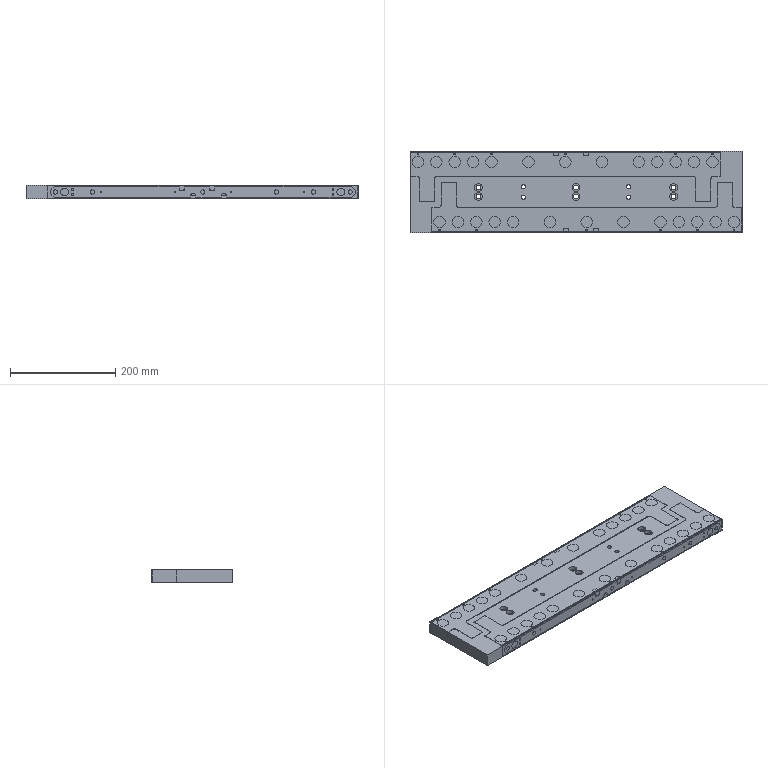NC program | NX | posted with a generic post | part box 631 x 154 x 25 mm
Lines 131 to 967 of 18383:
(HOLE_MILLING_COPY , TOOL : D10JING)
N242 T11 M6
N244 G54
N246 G17 G0 G90 X-200.5 Y47. B0. C0. S7000 M3
N248 G43 Z30. H11
N250 Z1.
N252 G94 G3 X-197.575 Y44.075 R2.925 F2000.
N254 X-194.65 Y47. R2.925
N256 X-194.65 Y47. Z0. I-5.85 J0.
N258 X-194.65 Y47. Z-1. I-5.85 J0.
N260 X-194.65 Y47. Z-2. I-5.85 J0.
N262 X-194.65 Y47. Z-3. I-5.85 J0.
N264 X-194.65 Y47. Z-4. I-5.85 J0.
N266 X-194.65 Y47. Z-5. I-5.85 J0.
N268 X-194.65 Y47. Z-6. I-5.85 J0.
N270 X-200.5 Y52.85 R5.85
N272 X-194.65 Y47. R-5.85
N274 X-197.575 Y49.925 R2.925
N276 X-200.5 Y47. R2.925
N278 G0 Z30.
N280 X-165.5
N282 Z1.
N284 G3 X-162.575 Y44.075 R2.925
N286 X-159.65 Y47. R2.925
N288 X-159.65 Y47. Z0. I-5.85 J0.
N290 X-159.65 Y47. Z-1. I-5.85 J0.
N292 X-159.65 Y47. Z-2. I-5.85 J0.
N294 X-159.65 Y47. Z-3. I-5.85 J0.
N296 X-159.65 Y47. Z-4. I-5.85 J0.
N298 X-159.65 Y47. Z-5. I-5.85 J0.
N300 X-159.65 Y47. Z-6. I-5.85 J0.
N302 X-165.5 Y52.85 R5.85
N304 X-159.65 Y47. R-5.85
N306 X-162.575 Y49.925 R2.925
N308 X-165.5 Y47. R2.925
N310 G0 Z30.
N312 X-130.5
N314 Z1.
N316 G3 X-127.575 Y44.075 R2.925
N318 X-124.65 Y47. R2.925
N320 X-124.65 Y47. Z0. I-5.85 J0.
N322 X-124.65 Y47. Z-1. I-5.85 J0.
N324 X-124.65 Y47. Z-2. I-5.85 J0.
N326 X-124.65 Y47. Z-3. I-5.85 J0.
N328 X-124.65 Y47. Z-4. I-5.85 J0.
N330 X-124.65 Y47. Z-5. I-5.85 J0.
N332 X-124.65 Y47. Z-6. I-5.85 J0.
N334 X-130.5 Y52.85 R5.85
N336 X-124.65 Y47. R-5.85
N338 X-127.575 Y49.925 R2.925
N340 X-130.5 Y47. R2.925
N342 G0 Z30.
N344 X-95.5
N346 Z1.
N348 G3 X-92.575 Y44.075 R2.925
N350 X-89.65 Y47. R2.925
N352 X-89.65 Y47. Z0. I-5.85 J0.
N354 X-89.65 Y47. Z-1. I-5.85 J0.
N356 X-89.65 Y47. Z-2. I-5.85 J0.
N358 X-89.65 Y47. Z-3. I-5.85 J0.
N360 X-89.65 Y47. Z-4. I-5.85 J0.
N362 X-89.65 Y47. Z-5. I-5.85 J0.
N364 X-89.65 Y47. Z-6. I-5.85 J0.
N366 X-95.5 Y52.85 R5.85
N368 X-89.65 Y47. R-5.85
N370 X-92.575 Y49.925 R2.925
N372 X-95.5 Y47. R2.925
N374 G0 Z30.
N376 X-60.5
N378 Z1.
N380 G3 X-57.575 Y44.075 R2.925
N382 X-54.65 Y47. R2.925
N384 X-54.65 Y47. Z0. I-5.85 J0.
N386 X-54.65 Y47. Z-1. I-5.85 J0.
N388 X-54.65 Y47. Z-2. I-5.85 J0.
N390 X-54.65 Y47. Z-3. I-5.85 J0.
N392 X-54.65 Y47. Z-4. I-5.85 J0.
N394 X-54.65 Y47. Z-5. I-5.85 J0.
N396 X-54.65 Y47. Z-6. I-5.85 J0.
N398 X-60.5 Y52.85 R5.85
N400 X-54.65 Y47. R-5.85
N402 X-57.575 Y49.925 R2.925
N404 X-60.5 Y47. R2.925
N406 G0 Z30.
N408 X9.5
N410 Z1.
N412 G3 X12.425 Y44.075 R2.925
N414 X15.35 Y47. R2.925
N416 X15.35 Y47. Z0. I-5.85 J0.
N418 X15.35 Y47. Z-1. I-5.85 J0.
N420 X15.35 Y47. Z-2. I-5.85 J0.
N422 X15.35 Y47. Z-3. I-5.85 J0.
N424 X15.35 Y47. Z-4. I-5.85 J0.
N426 X15.35 Y47. Z-5. I-5.85 J0.
N428 X15.35 Y47. Z-6. I-5.85 J0.
N430 X9.5 Y52.85 R5.85
N432 X15.35 Y47. R-5.85
N434 X12.425 Y49.925 R2.925
N436 X9.5 Y47. R2.925
N438 G0 Z30.
N440 X79.5
N442 Z1.
N444 G3 X82.425 Y44.075 R2.925
N446 X85.35 Y47. R2.925
N448 X85.35 Y47. Z0. I-5.85 J0.
N450 X85.35 Y47. Z-1. I-5.85 J0.
N452 X85.35 Y47. Z-2. I-5.85 J0.
N454 X85.35 Y47. Z-3. I-5.85 J0.
N456 X85.35 Y47. Z-4. I-5.85 J0.
N458 X85.35 Y47. Z-5. I-5.85 J0.
N460 X85.35 Y47. Z-6. I-5.85 J0.
N462 X79.5 Y52.85 R5.85
N464 X85.35 Y47. R-5.85
N466 X82.425 Y49.925 R2.925
N468 X79.5 Y47. R2.925
N470 G0 Z30.
N472 X149.5
N474 Z1.
N476 G3 X152.425 Y44.075 R2.925
N478 X155.35 Y47. R2.925
N480 X155.35 Y47. Z0. I-5.85 J0.
N482 X155.35 Y47. Z-1. I-5.85 J0.
N484 X155.35 Y47. Z-2. I-5.85 J0.
N486 X155.35 Y47. Z-3. I-5.85 J0.
N488 X155.35 Y47. Z-4. I-5.85 J0.
N490 X155.35 Y47. Z-5. I-5.85 J0.
N492 X155.35 Y47. Z-6. I-5.85 J0.
N494 X149.5 Y52.85 R5.85
N496 X155.35 Y47. R-5.85
N498 X152.425 Y49.925 R2.925
N500 X149.5 Y47. R2.925
N502 G0 Z30.
N504 X219.5
N506 Z1.
N508 G3 X222.425 Y44.075 R2.925
N510 X225.35 Y47. R2.925
N512 X225.35 Y47. Z0. I-5.85 J0.
N514 X225.35 Y47. Z-1. I-5.85 J0.
N516 X225.35 Y47. Z-2. I-5.85 J0.
N518 X225.35 Y47. Z-3. I-5.85 J0.
N520 X225.35 Y47. Z-4. I-5.85 J0.
N522 X225.35 Y47. Z-5. I-5.85 J0.
N524 X225.35 Y47. Z-6. I-5.85 J0.
N526 X219.5 Y52.85 R5.85
N528 X225.35 Y47. R-5.85
N530 X222.425 Y49.925 R2.925
N532 X219.5 Y47. R2.925
N534 G0 Z30.
N536 X254.5
N538 Z1.
N540 G3 X257.425 Y44.075 R2.925
N542 X260.35 Y47. R2.925
N544 X260.35 Y47. Z0. I-5.85 J0.
N546 X260.35 Y47. Z-1. I-5.85 J0.
N548 X260.35 Y47. Z-2. I-5.85 J0.
N550 X260.35 Y47. Z-3. I-5.85 J0.
N552 X260.35 Y47. Z-4. I-5.85 J0.
N554 X260.35 Y47. Z-5. I-5.85 J0.
N556 X260.35 Y47. Z-6. I-5.85 J0.
N558 X254.5 Y52.85 R5.85
N560 X260.35 Y47. R-5.85
N562 X257.425 Y49.925 R2.925
N564 X254.5 Y47. R2.925
N566 G0 Z30.
N568 X289.5
N570 Z1.
N572 G3 X292.425 Y44.075 R2.925
N574 X295.35 Y47. R2.925
N576 X295.35 Y47. Z0. I-5.85 J0.
N578 X295.35 Y47. Z-1. I-5.85 J0.
N580 X295.35 Y47. Z-2. I-5.85 J0.
N582 X295.35 Y47. Z-3. I-5.85 J0.
N584 X295.35 Y47. Z-4. I-5.85 J0.
N586 X295.35 Y47. Z-5. I-5.85 J0.
N588 X295.35 Y47. Z-6. I-5.85 J0.
N590 X289.5 Y52.85 R5.85
N592 X295.35 Y47. R-5.85
N594 X292.425 Y49.925 R2.925
N596 X289.5 Y47. R2.925
N598 G0 Z30.
N600 X324.5
N602 Z1.
N604 G3 X327.425 Y44.075 R2.925
N606 X330.35 Y47. R2.925
N608 X330.35 Y47. Z0. I-5.85 J0.
N610 X330.35 Y47. Z-1. I-5.85 J0.
N612 X330.35 Y47. Z-2. I-5.85 J0.
N614 X330.35 Y47. Z-3. I-5.85 J0.
N616 X330.35 Y47. Z-4. I-5.85 J0.
N618 X330.35 Y47. Z-5. I-5.85 J0.
N620 X330.35 Y47. Z-6. I-5.85 J0.
N622 X324.5 Y52.85 R5.85
N624 X330.35 Y47. R-5.85
N626 X327.425 Y49.925 R2.925
N628 X324.5 Y47. R2.925
N630 G0 Z30.
N632 X359.5
N634 Z1.
N636 G3 X362.425 Y44.075 R2.925
N638 X365.35 Y47. R2.925
N640 X365.35 Y47. Z0. I-5.85 J0.
N642 X365.35 Y47. Z-1. I-5.85 J0.
N644 X365.35 Y47. Z-2. I-5.85 J0.
N646 X365.35 Y47. Z-3. I-5.85 J0.
N648 X365.35 Y47. Z-4. I-5.85 J0.
N650 X365.35 Y47. Z-5. I-5.85 J0.
N652 X365.35 Y47. Z-6. I-5.85 J0.
N654 X359.5 Y52.85 R5.85
N656 X365.35 Y47. R-5.85
N658 X362.425 Y49.925 R2.925
N660 X359.5 Y47. R2.925
N662 G0 Z30.
N664 X400.5 Y-67.
N666 Z1.
N668 G3 X403.425 Y-69.925 R2.925
N670 X406.35 Y-67. R2.925
N672 X406.35 Y-67. Z0. I-5.85 J0.
N674 X406.35 Y-67. Z-1. I-5.85 J0.
N676 X406.35 Y-67. Z-2. I-5.85 J0.
N678 X406.35 Y-67. Z-3. I-5.85 J0.
N680 X406.35 Y-67. Z-4. I-5.85 J0.
N682 X406.35 Y-67. Z-5. I-5.85 J0.
N684 X406.35 Y-67. Z-6. I-5.85 J0.
N686 X400.5 Y-61.15 R5.85
N688 X406.35 Y-67. R-5.85
N690 X403.425 Y-64.075 R2.925
N692 X400.5 Y-67. R2.925
N694 G0 Z30.
N696 X365.5
N698 Z1.
N700 G3 X368.425 Y-69.925 R2.925
N702 X371.35 Y-67. R2.925
N704 X371.35 Y-67. Z0. I-5.85 J0.
N706 X371.35 Y-67. Z-1. I-5.85 J0.
N708 X371.35 Y-67. Z-2. I-5.85 J0.
N710 X371.35 Y-67. Z-3. I-5.85 J0.
N712 X371.35 Y-67. Z-4. I-5.85 J0.
N714 X371.35 Y-67. Z-5. I-5.85 J0.
N716 X371.35 Y-67. Z-6. I-5.85 J0.
N718 X365.5 Y-61.15 R5.85
N720 X371.35 Y-67. R-5.85
N722 X368.425 Y-64.075 R2.925
N724 X365.5 Y-67. R2.925
N726 G0 Z30.
N728 X330.5
N730 Z1.
N732 G3 X333.425 Y-69.925 R2.925
N734 X336.35 Y-67. R2.925
N736 X336.35 Y-67. Z0. I-5.85 J0.
N738 X336.35 Y-67. Z-1. I-5.85 J0.
N740 X336.35 Y-67. Z-2. I-5.85 J0.
N742 X336.35 Y-67. Z-3. I-5.85 J0.
N744 X336.35 Y-67. Z-4. I-5.85 J0.
N746 X336.35 Y-67. Z-5. I-5.85 J0.
N748 X336.35 Y-67. Z-6. I-5.85 J0.
N750 X330.5 Y-61.15 R5.85
N752 X336.35 Y-67. R-5.85
N754 X333.425 Y-64.075 R2.925
N756 X330.5 Y-67. R2.925
N758 G0 Z30.
N760 X295.5
N762 Z1.
N764 G3 X298.425 Y-69.925 R2.925
N766 X301.35 Y-67. R2.925
N768 X301.35 Y-67. Z0. I-5.85 J0.
N770 X301.35 Y-67. Z-1. I-5.85 J0.
N772 X301.35 Y-67. Z-2. I-5.85 J0.
N774 X301.35 Y-67. Z-3. I-5.85 J0.
N776 X301.35 Y-67. Z-4. I-5.85 J0.
N778 X301.35 Y-67. Z-5. I-5.85 J0.
N780 X301.35 Y-67. Z-6. I-5.85 J0.
N782 X295.5 Y-61.15 R5.85
N784 X301.35 Y-67. R-5.85
N786 X298.425 Y-64.075 R2.925
N788 X295.5 Y-67. R2.925
N790 G0 Z30.
N792 X260.5
N794 Z1.
N796 G3 X263.425 Y-69.925 R2.925
N798 X266.35 Y-67. R2.925
N800 X266.35 Y-67. Z0. I-5.85 J0.
N802 X266.35 Y-67. Z-1. I-5.85 J0.
N804 X266.35 Y-67. Z-2. I-5.85 J0.
N806 X266.35 Y-67. Z-3. I-5.85 J0.
N808 X266.35 Y-67. Z-4. I-5.85 J0.
N810 X266.35 Y-67. Z-5. I-5.85 J0.
N812 X266.35 Y-67. Z-6. I-5.85 J0.
N814 X260.5 Y-61.15 R5.85
N816 X266.35 Y-67. R-5.85
N818 X263.425 Y-64.075 R2.925
N820 X260.5 Y-67. R2.925
N822 G0 Z30.
N824 X190.5
N826 Z1.
N828 G3 X193.425 Y-69.925 R2.925
N830 X196.35 Y-67. R2.925
N832 X196.35 Y-67. Z0. I-5.85 J0.
N834 X196.35 Y-67. Z-1. I-5.85 J0.
N836 X196.35 Y-67. Z-2. I-5.85 J0.
N838 X196.35 Y-67. Z-3. I-5.85 J0.
N840 X196.35 Y-67. Z-4. I-5.85 J0.
N842 X196.35 Y-67. Z-5. I-5.85 J0.
N844 X196.35 Y-67. Z-6. I-5.85 J0.
N846 X190.5 Y-61.15 R5.85
N848 X196.35 Y-67. R-5.85
N850 X193.425 Y-64.075 R2.925
N852 X190.5 Y-67. R2.925
N854 G0 Z30.
N856 X120.5
N858 Z1.
N860 G3 X123.425 Y-69.925 R2.925
N862 X126.35 Y-67. R2.925
N864 X126.35 Y-67. Z0. I-5.85 J0.
N866 X126.35 Y-67. Z-1. I-5.85 J0.
N868 X126.35 Y-67. Z-2. I-5.85 J0.
N870 X126.35 Y-67. Z-3. I-5.85 J0.
N872 X126.35 Y-67. Z-4. I-5.85 J0.
N874 X126.35 Y-67. Z-5. I-5.85 J0.
N876 X126.35 Y-67. Z-6. I-5.85 J0.
N878 X120.5 Y-61.15 R5.85
N880 X126.35 Y-67. R-5.85
N882 X123.425 Y-64.075 R2.925
N884 X120.5 Y-67. R2.925
N886 G0 Z30.
N888 X50.5
N890 Z1.
N892 G3 X53.425 Y-69.925 R2.925
N894 X56.35 Y-67. R2.925
N896 X56.35 Y-67. Z0. I-5.85 J0.
N898 X56.35 Y-67. Z-1. I-5.85 J0.
N900 X56.35 Y-67. Z-2. I-5.85 J0.
N902 X56.35 Y-67. Z-3. I-5.85 J0.
N904 X56.35 Y-67. Z-4. I-5.85 J0.
N906 X56.35 Y-67. Z-5. I-5.85 J0.
N908 X56.35 Y-67. Z-6. I-5.85 J0.
N910 X50.5 Y-61.15 R5.85
N912 X56.35 Y-67. R-5.85
N914 X53.425 Y-64.075 R2.925
N916 X50.5 Y-67. R2.925
N918 G0 Z30.
N920 X-19.5
N922 Z1.
N924 G3 X-16.575 Y-69.925 R2.925
N926 X-13.65 Y-67. R2.925
N928 X-13.65 Y-67. Z0. I-5.85 J0.
N930 X-13.65 Y-67. Z-1. I-5.85 J0.
N932 X-13.65 Y-67. Z-2. I-5.85 J0.
N934 X-13.65 Y-67. Z-3. I-5.85 J0.
N936 X-13.65 Y-67. Z-4. I-5.85 J0.
N938 X-13.65 Y-67. Z-5. I-5.85 J0.
N940 X-13.65 Y-67. Z-6. I-5.85 J0.
N942 X-19.5 Y-61.15 R5.85
N944 X-13.65 Y-67. R-5.85
N946 X-16.575 Y-64.075 R2.925
N948 X-19.5 Y-67. R2.925
N950 G0 Z30.
N952 X-54.5
N954 Z1.
N956 G3 X-51.575 Y-69.925 R2.925
N958 X-48.65 Y-67. R2.925
N960 X-48.65 Y-67. Z0. I-5.85 J0.
N962 X-48.65 Y-67. Z-1. I-5.85 J0.
N964 X-48.65 Y-67. Z-2. I-5.85 J0.
N966 X-48.65 Y-67. Z-3. I-5.85 J0.
N968 X-48.65 Y-67. Z-4. I-5.85 J0.
N970 X-48.65 Y-67. Z-5. I-5.85 J0.
N972 X-48.65 Y-67. Z-6. I-5.85 J0.
N974 X-54.5 Y-61.15 R5.85
N976 X-48.65 Y-67. R-5.85
N978 X-51.575 Y-64.075 R2.925
N980 X-54.5 Y-67. R2.925
N982 G0 Z30.
N984 X-89.5
N986 Z1.
N988 G3 X-86.575 Y-69.925 R2.925
N990 X-83.65 Y-67. R2.925
N992 X-83.65 Y-67. Z0. I-5.85 J0.
N994 X-83.65 Y-67. Z-1. I-5.85 J0.
N996 X-83.65 Y-67. Z-2. I-5.85 J0.
N998 X-83.65 Y-67. Z-3. I-5.85 J0.
N1000 X-83.65 Y-67. Z-4. I-5.85 J0.
N1002 X-83.65 Y-67. Z-5. I-5.85 J0.
N1004 X-83.65 Y-67. Z-6. I-5.85 J0.
N1006 X-89.5 Y-61.15 R5.85
N1008 X-83.65 Y-67. R-5.85
N1010 X-86.575 Y-64.075 R2.925
N1012 X-89.5 Y-67. R2.925
N1014 G0 Z30.
N1016 X-124.5
N1018 Z1.
N1020 G3 X-121.575 Y-69.925 R2.925
N1022 X-118.65 Y-67. R2.925
N1024 X-118.65 Y-67. Z0. I-5.85 J0.
N1026 X-118.65 Y-67. Z-1. I-5.85 J0.
N1028 X-118.65 Y-67. Z-2. I-5.85 J0.
N1030 X-118.65 Y-67. Z-3. I-5.85 J0.
N1032 X-118.65 Y-67. Z-4. I-5.85 J0.
N1034 X-118.65 Y-67. Z-5. I-5.85 J0.
N1036 X-118.65 Y-67. Z-6. I-5.85 J0.
N1038 X-124.5 Y-61.15 R5.85
N1040 X-118.65 Y-67. R-5.85
N1042 X-121.575 Y-64.075 R2.925
N1044 X-124.5 Y-67. R2.925
N1046 G0 Z30.
N1048 X-159.5
N1050 Z1.
N1052 G3 X-156.575 Y-69.925 R2.925
N1054 X-153.65 Y-67. R2.925
N1056 X-153.65 Y-67. Z0. I-5.85 J0.
N1058 X-153.65 Y-67. Z-1. I-5.85 J0.
N1060 X-153.65 Y-67. Z-2. I-5.85 J0.
N1062 X-153.65 Y-67. Z-3. I-5.85 J0.
N1064 X-153.65 Y-67. Z-4. I-5.85 J0.
N1066 X-153.65 Y-67. Z-5. I-5.85 J0.
N1068 X-153.65 Y-67. Z-6. I-5.85 J0.
N1070 X-159.5 Y-61.15 R5.85
N1072 X-153.65 Y-67. R-5.85
N1074 X-156.575 Y-64.075 R2.925
N1076 X-159.5 Y-67. R2.925
N1078 G0 Z30.
(ZLEVEL_PROFILE_COPY_3 , TOOL : D10JING)
N1080 X152.468 Y46.555
N1082 Z-4.5
N1084 G1 X152.5 Y46.757 Z-4.511 F1000.
N1086 Y47.002 Z-4.524
N1088 Y47.247 Z-4.536
N1090 X152.427 Y47.701 Z-4.56
N1092 X152.287 Y48.138 Z-4.585
N1094 X152.065 Y48.575 Z-4.61
N1096 X151.904 Y48.812 Z-4.625
N1098 X151.741 Y48.995 Z-4.638
N1100 X151.729 Y48.997 Z-4.639
N1102 X151.497 Y49.229 Z-4.656
N1104 X151.496 Y49.24
N1106 X151.313 Y49.403 Z-4.669
N1108 X151.077 Y49.564 Z-4.684
N1110 X150.857 Y49.676 Z-4.697
N1112 X150.638 Y49.786 Z-4.71
N1114 X150.08 Y49.954 Z-4.741
N1116 X149.501 Y50.01 Z-4.771
N1118 X148.921 Y49.954 Z-4.802
N1120 X148.363 Y49.787 Z-4.832
N1122 X148.143 Y49.676 Z-4.845
N1124 X147.925 Y49.565 Z-4.858
N1126 X147.688 Y49.404 Z-4.873
N1128 X147.505 Y49.241 Z-4.886
N1130 X147.503 Y49.229
N1132 X147.32 Y49.065 Z-4.899
N1134 X146.936 Y48.562 Z-4.932
N1136 X146.826 Y48.343 Z-4.945
N1138 X146.816 Y48.34 Z-4.946
N1140 X146.706 Y48.121 Z-4.959
N1142 X146.571 Y47.692 Z-4.982
N1144 X146.5 Y47.247 Z-5.006
N1146 Y47.002 Z-5.019
N1148 Y46.757 Z-5.031
N1150 X146.57 Y46.31 Z-5.055
N1152 X146.706 Y45.879 Z-5.079
N1154 X146.816 Y45.66 Z-5.092
N1156 X146.826 Y45.658
N1158 X146.936 Y45.439 Z-5.105
N1160 X147.215 Y45.053 Z-5.13
N1162 X147.553 Y44.715 Z-5.155
N1164 X147.939 Y44.436 Z-5.18
N1166 X148.158 Y44.326 Z-5.193
N1168 X148.16 Y44.316
N1170 X148.379 Y44.206 Z-5.206
N1172 X148.957 Y44.039 Z-5.238
N1174 X149.557 Y43.991 Z-5.269
N1176 X150.154 Y44.062 Z-5.301
N1178 X150.725 Y44.25 Z-5.332
N1180 X151.247 Y44.549 Z-5.364
N1182 X151.699 Y44.945 Z-5.395
N1184 X152.064 Y45.423 Z-5.427
N1186 X152.286 Y45.861 Z-5.453
N1188 X152.428 Y46.301 Z-5.477
N1190 X152.5 Y46.757 Z-5.501
N1192 Y47.002 Z-5.514
N1194 Y47.247 Z-5.527
N1196 X152.427 Y47.701 Z-5.551
N1198 X152.287 Y48.138 Z-5.575
N1200 X152.065 Y48.575 Z-5.601
N1202 X151.904 Y48.812 Z-5.616
N1204 X151.741 Y48.995 Z-5.628
N1206 X151.729 Y48.997 Z-5.629
N1208 X151.497 Y49.229 Z-5.646
N1210 X151.496 Y49.24 Z-5.647
N1212 X151.313 Y49.403 Z-5.66
N1214 X151.077 Y49.564 Z-5.675
N1216 X150.857 Y49.676 Z-5.688
N1218 X150.638 Y49.786 Z-5.7
N1220 X150.08 Y49.954 Z-5.731
N1222 X149.501 Y50.01 Z-5.761
N1224 X148.921 Y49.954 Z-5.792
N1226 X148.363 Y49.787 Z-5.822
N1228 X148.143 Y49.676 Z-5.835
N1230 X147.925 Y49.565 Z-5.848
N1232 X147.688 Y49.404 Z-5.863
N1234 X147.505 Y49.241 Z-5.876
N1236 X147.503 Y49.229 Z-5.877
N1238 X147.32 Y49.065 Z-5.89
N1240 X146.936 Y48.562 Z-5.923
N1242 X146.826 Y48.343 Z-5.936
N1244 X146.816 Y48.34
N1246 X146.706 Y48.121 Z-5.949
N1248 X146.571 Y47.692 Z-5.973
N1250 X146.5 Y47.247 Z-5.996
N1252 Y47.002 Z-6.009
N1254 Y46.757 Z-6.022
N1256 X146.57 Y46.31 Z-6.046
N1258 X146.706 Y45.879 Z-6.069
N1260 X146.816 Y45.66 Z-6.082
N1262 X146.826 Y45.658 Z-6.083
N1264 X146.936 Y45.439 Z-6.095
N1266 X147.215 Y45.053 Z-6.12
N1268 X147.553 Y44.715 Z-6.145
N1270 X147.939 Y44.436 Z-6.17
N1272 X148.158 Y44.326 Z-6.183
N1274 X148.16 Y44.316 Z-6.184
N1276 X148.379 Y44.206 Z-6.197
N1278 X148.957 Y44.039 Z-6.228
N1280 X149.557 Y43.991 Z-6.26
N1282 X150.154 Y44.062 Z-6.291
N1284 X150.725 Y44.25 Z-6.323
N1286 X151.247 Y44.549 Z-6.354
N1288 X151.699 Y44.945 Z-6.386
N1290 X152.064 Y45.423 Z-6.417
N1292 X152.286 Y45.861 Z-6.443
N1294 X152.428 Y46.301 Z-6.467
N1296 X152.5 Y46.757 Z-6.491
N1298 Y47.002 Z-6.504
N1300 Y47.247 Z-6.517
N1302 X152.427 Y47.701 Z-6.541
N1304 X152.287 Y48.138 Z-6.565
N1306 X152.065 Y48.575 Z-6.591
N1308 X151.904 Y48.812 Z-6.606
N1310 X151.741 Y48.995 Z-6.619
N1312 X151.729 Y48.997
N1314 X151.497 Y49.229 Z-6.637
N1316 X151.496 Y49.24
N1318 X151.313 Y49.403 Z-6.65
N1320 X151.077 Y49.564 Z-6.665
N1322 X150.857 Y49.676 Z-6.678
N1324 X150.638 Y49.786 Z-6.691
N1326 X150.08 Y49.954 Z-6.721
N1328 X149.501 Y50.01 Z-6.752
N1330 X148.921 Y49.954 Z-6.782
N1332 X148.363 Y49.787 Z-6.813
N1334 X148.143 Y49.676 Z-6.826
N1336 X147.925 Y49.565 Z-6.839
N1338 X147.688 Y49.404 Z-6.854
N1340 X147.505 Y49.241 Z-6.866
N1342 X147.503 Y49.229 Z-6.867
N1344 X147.32 Y49.065 Z-6.88
N1346 X146.936 Y48.562 Z-6.913
N1348 X146.826 Y48.343 Z-6.926
N1350 X146.816 Y48.34 Z-6.927
N1352 X146.706 Y48.121 Z-6.939
N1354 X146.571 Y47.692 Z-6.963
N1356 X146.5 Y47.247 Z-6.987
N1358 Y47.002 Z-6.999
N1360 Y46.757 Z-7.012
N1362 X146.57 Y46.31 Z-7.036
N1364 X146.706 Y45.879 Z-7.06
N1366 X146.816 Y45.66 Z-7.072
N1368 X146.826 Y45.658 Z-7.073
N1370 X146.936 Y45.439 Z-7.086
N1372 X147.215 Y45.053 Z-7.111
N1374 X147.553 Y44.715 Z-7.136
N1376 X147.939 Y44.436 Z-7.161
N1378 X148.158 Y44.326 Z-7.174
N1380 X148.16 Y44.316
N1382 X148.379 Y44.206 Z-7.187
N1384 X148.957 Y44.039 Z-7.219
N1386 X149.557 Y43.991 Z-7.25
N1388 X150.154 Y44.062 Z-7.282
N1390 X150.725 Y44.25 Z-7.313
N1392 X151.247 Y44.549 Z-7.345
N1394 X151.699 Y44.945 Z-7.376
N1396 X152.064 Y45.423 Z-7.408
N1398 X152.286 Y45.861 Z-7.433
N1400 X152.428 Y46.301 Z-7.458
N1402 X152.5 Y46.757 Z-7.482
N1404 Y47.002 Z-7.495
N1406 Y47.247 Z-7.507
N1408 X152.427 Y47.701 Z-7.532
N1410 X152.287 Y48.138 Z-7.556
N1412 X152.065 Y48.575 Z-7.581
N1414 X151.904 Y48.812 Z-7.596
N1416 X151.741 Y48.995 Z-7.609
N1418 X151.729 Y48.997 Z-7.61
N1420 X151.497 Y49.229 Z-7.627
N1422 X151.496 Y49.24 Z-7.628
N1424 X151.313 Y49.403 Z-7.64
N1426 X151.077 Y49.564 Z-7.655
N1428 X150.857 Y49.676 Z-7.668
N1430 X150.638 Y49.786 Z-7.681
N1432 X150.08 Y49.954 Z-7.712
N1434 X149.501 Y50.01 Z-7.742
N1436 X148.921 Y49.954 Z-7.773
N1438 X148.363 Y49.787 Z-7.803
N1440 X148.143 Y49.676 Z-7.816
N1442 X147.925 Y49.565 Z-7.829
N1444 X147.688 Y49.404 Z-7.844
N1446 X147.505 Y49.241 Z-7.857
N1448 X147.504 Y49.235
N1450 X147.503 Y49.229 F1500.
N1452 G3 X146.826 Y48.343 R3.008
N1454 G1 X146.816 Y48.34
N1456 G3 X146.816 Y45.66 R3.
N1458 G1 X146.826 Y45.658
N1460 G3 X148.158 Y44.326 R2.998
N1462 G1 X148.16 Y44.316
N1464 G3 X151.741 Y48.995 R3.
N1466 G1 X151.729 Y48.997
N1468 X151.497 Y49.229
N1470 X151.496 Y49.24
N1472 G3 X147.505 Y49.241 R3.
N1474 G1 X147.504 Y49.235
N1476 X147.347 Y49.078 Z-7.886
N1478 X147.2 Y48.916 Z-7.915
N1480 X147.067 Y48.74 Z-7.944
N1482 X146.946 Y48.555 Z-7.973
N1484 X146.836 Y48.365 Z-8.002
N1486 X146.744 Y48.167 Z-8.031
N1488 X146.667 Y47.961 Z-8.06
N1490 X146.604 Y47.749 Z-8.089
N1492 X146.555 Y47.535 Z-8.118
N1494 X146.524 Y47.317 Z-8.147
N1496 X146.509 Y47.096 Z-8.176
N1498 X146.503 Y46.876 Z-8.205
N1500 X146.527 Y46.657 Z-8.234
N1502 X146.56 Y46.439 Z-8.263
N1504 X146.611 Y46.224 Z-8.292
N1506 X146.676 Y46.014 Z-8.321
N1508 X146.755 Y45.81 Z-8.35
N1510 X146.847 Y45.612 Z-8.379
N1512 X146.959 Y45.421 Z-8.408
N1514 X147.083 Y45.239 Z-8.438
N1516 X147.218 Y45.064 Z-8.467
N1518 X147.367 Y44.9 Z-8.496
N1520 X147.529 Y44.75 Z-8.525
N1522 X147.7 Y44.611 Z-8.554
N1524 X147.88 Y44.483 Z-8.583
N1526 X148.07 Y44.37 Z-8.612
N1528 X148.266 Y44.274 Z-8.641
N1530 X148.469 Y44.192 Z-8.67
N1532 X148.678 Y44.122 Z-8.699
N1534 X148.892 Y44.069 Z-8.728
N1536 X149.109 Y44.034 Z-8.757
N1538 X149.329 Y44.013 Z-8.786
N1540 X149.549 Y44.007 Z-8.815
N1542 X149.769 Y44.019 Z-8.844
N1544 X149.987 Y44.048 Z-8.873
N1546 X150.203 Y44.092 Z-8.902
N1548 X150.416 Y44.15 Z-8.931
N1550 X150.623 Y44.225 Z-8.96
N1552 X150.823 Y44.317 Z-8.989
N1554 X151.017 Y44.422 Z-9.018
N1556 X151.204 Y44.539 Z-9.047
N1558 X151.38 Y44.671 Z-9.076
N1560 X151.545 Y44.817 Z-9.105
N1562 X151.7 Y44.973 Z-9.134
N1564 X151.845 Y45.139 Z-9.163
N1566 X151.975 Y45.317 Z-9.192
N1568 X152.091 Y45.505 Z-9.221
N1570 X152.194 Y45.699 Z-9.25
N1572 X152.284 Y45.9 Z-9.279
N1574 X152.357 Y46.108 Z-9.308
N1576 X152.414 Y46.321 Z-9.337
N1578 X152.455 Y46.537 Z-9.366
N1580 X152.484 Y46.756 Z-9.395
N1582 X152.493 Y46.976 Z-9.424
N1584 X152.485 Y47.196 Z-9.453
N1586 X152.462 Y47.415 Z-9.482
N1588 X152.426 Y47.633 Z-9.511
N1590 X152.371 Y47.846 Z-9.54
N1592 X152.3 Y48.055 Z-9.569
N1594 X152.214 Y48.258 Z-9.598
N1596 X152.116 Y48.455 Z-9.627
N1598 X152.002 Y48.643 Z-9.656
N1600 X151.872 Y48.822 Z-9.685
N1602 X151.737 Y48.995 Z-9.714
N1604 X151.729 Y48.997
N1606 X151.497 Y49.229
N1608 X151.496 Y49.24
N1610 G3 X147.505 Y49.241 R3.
N1612 G1 X147.504 Y49.235
N1614 X147.347 Y49.078 Z-9.743
N1616 X147.2 Y48.916 Z-9.772
N1618 X147.066 Y48.741 Z-9.801
N1620 X146.944 Y48.556 Z-9.83
N1622 X146.837 Y48.365 Z-9.859
N1624 X146.744 Y48.167 Z-9.888
N1626 X146.667 Y47.961 Z-9.917
N1628 X146.604 Y47.75 Z-9.946
N1630 X146.555 Y47.535 Z-9.975
N1632 X146.524 Y47.317 Z-10.004
N1634 X146.509 Y47.096 Z-10.033
N1636 X146.503 Y46.876 Z-10.063
N1638 X146.528 Y46.657 Z-10.092
N1640 X146.56 Y46.439 Z-10.121
N1642 X146.611 Y46.224 Z-10.15
N1644 X146.676 Y46.014 Z-10.179
N1646 X146.754 Y45.808 Z-10.208
N1648 X146.849 Y45.609 Z-10.237
N1650 X146.96 Y45.419 Z-10.266
N1652 X147.084 Y45.236 Z-10.295
N1654 X147.22 Y45.062 Z-10.324
N1656 X147.368 Y44.898 Z-10.353
N1658 X147.53 Y44.748 Z-10.382
N1660 X147.703 Y44.609 Z-10.411
N1662 X147.883 Y44.482 Z-10.44
N1664 X148.072 Y44.368 Z-10.469
N1666 X148.27 Y44.272 Z-10.498
N1668 X148.475 Y44.19 Z-10.527
N1670 X148.684 Y44.121 Z-10.556
N1672 X148.897 Y44.066 Z-10.585
N1674 X149.115 Y44.032 Z-10.614
N1676 X149.335 Y44.013 Z-10.643
N1678 X149.555 Y44.008 Z-10.672
N1680 X149.775 Y44.018 Z-10.701
N1682 X149.993 Y44.048 Z-10.73
N1684 X150.209 Y44.094 Z-10.759
N1686 X150.421 Y44.153 Z-10.788
N1688 X150.629 Y44.226 Z-10.817
N1690 X150.829 Y44.319 Z-10.846
N1692 X151.022 Y44.425 Z-10.875
N1694 X151.208 Y44.543 Z-10.904
N1696 X151.386 Y44.673 Z-10.933
N1698 X151.55 Y44.82 Z-10.962
N1700 X151.704 Y44.978 Z-10.991
N1702 X151.848 Y45.145 Z-11.02
N1704 X151.98 Y45.321 Z-11.049
N1706 X152.095 Y45.509 Z-11.078
N1708 X152.196 Y45.705 Z-11.107
N1710 X152.285 Y45.906 Z-11.136
N1712 X152.361 Y46.113 Z-11.165
N1714 X152.416 Y46.327 Z-11.194
N1716 X152.456 Y46.543 Z-11.223
N1718 X152.483 Y46.762 Z-11.252
N1720 X152.495 Y46.982 Z-11.281
N1722 X152.486 Y47.202 Z-11.31
N1724 X152.462 Y47.421 Z-11.339
N1726 X152.424 Y47.639 Z-11.368
N1728 X152.371 Y47.853 Z-11.397
N1730 X152.298 Y48.06 Z-11.426
N1732 X152.212 Y48.263 Z-11.455
N1734 X152.112 Y48.46 Z-11.484
N1736 X152. Y48.649 Z-11.513
N1738 X151.869 Y48.828 Z-11.542
N1740 X151.732 Y48.997 Z-11.571
N1742 X151.729
N1744 X151.497 Y49.229
N1746 X151.496 Y49.24
N1748 G3 X147.505 Y49.241 R3.
N1750 G1 X147.504 Y49.235
N1752 X147.347 Y49.078 Z-11.6
N1754 X147.2 Y48.916 Z-11.629
N1756 X147.066 Y48.741 Z-11.658
N1758 X146.944 Y48.556 Z-11.688
N1760 X146.837 Y48.365 Z-11.717
N1762 X146.744 Y48.167 Z-11.746
N1764 X146.667 Y47.961 Z-11.775
N1766 X146.604 Y47.75 Z-11.804
N1768 X146.555 Y47.535 Z-11.833
N1770 X146.524 Y47.317 Z-11.862
N1772 X146.509 Y47.097 Z-11.891
N1774 X146.503 Y46.876 Z-11.92
N1776 X146.528 Y46.657 Z-11.949
N1778 X146.56 Y46.439 Z-11.978
N1780 X146.611 Y46.225 Z-12.007
N1782 X146.676 Y46.014 Z-12.036
N1784 X146.754 Y45.808 Z-12.065
N1786 X146.849 Y45.609 Z-12.094
N1788 X146.96 Y45.419 Z-12.123
N1790 X147.084 Y45.236 Z-12.152
N1792 X147.22 Y45.062 Z-12.181
N1794 X147.368 Y44.898 Z-12.21
N1796 X147.53 Y44.748 Z-12.239
N1798 X147.703 Y44.61 Z-12.268
N1800 X147.883 Y44.482 Z-12.297
N1802 X148.072 Y44.368 Z-12.326
N1804 X148.27 Y44.272 Z-12.355
N1806 X148.475 Y44.19 Z-12.384
N1808 X148.684 Y44.121 Z-12.413
N1810 X148.897 Y44.066 Z-12.442
N1812 X149.115 Y44.032 Z-12.471
N1814 X149.335 Y44.013 Z-12.5
N1816 X149.555 Y44.008 Z-12.529
N1818 X149.775 Y44.018 Z-12.558
N1820 X149.993 Y44.048 Z-12.587
N1822 X150.209 Y44.094 Z-12.616
N1824 X150.421 Y44.153 Z-12.645
N1826 X150.629 Y44.226 Z-12.674
N1828 X150.829 Y44.319 Z-12.703
N1830 X151.022 Y44.425 Z-12.732
N1832 X151.208 Y44.543 Z-12.761
N1834 X151.386 Y44.673 Z-12.79
N1836 X151.55 Y44.82 Z-12.819
N1838 X151.704 Y44.978 Z-12.848
N1840 X151.848 Y45.145 Z-12.877
N1842 X151.98 Y45.321 Z-12.906
N1844 X152.095 Y45.509 Z-12.935
N1846 X152.196 Y45.705 Z-12.964
N1848 X152.285 Y45.906 Z-12.993
N1850 X152.361 Y46.114 Z-13.022
N1852 X152.416 Y46.327 Z-13.051
N1854 X152.456 Y46.543 Z-13.08
N1856 X152.483 Y46.762 Z-13.109
N1858 X152.495 Y46.982 Z-13.138
N1860 X152.486 Y47.202 Z-13.167
N1862 X152.462 Y47.421 Z-13.196
N1864 X152.424 Y47.639 Z-13.225
N1866 X152.371 Y47.853 Z-13.254
N1868 X152.298 Y48.06 Z-13.283
N1870 X152.212 Y48.263 Z-13.313
N1872 X152.112 Y48.46 Z-13.342
N1874 X152. Y48.649 Z-13.371
N1876 X151.869 Y48.828 Z-13.4
N1878 X151.732 Y48.997 Z-13.429
N1880 X151.729
N1882 X151.497 Y49.229
N1884 X151.496 Y49.24
N1886 G3 X147.505 Y49.241 R3.
N1888 G1 X147.504 Y49.235
N1890 X147.346 Y49.078 Z-13.458
N1892 X147.2 Y48.916 Z-13.487
N1894 X147.066 Y48.741 Z-13.516
N1896 X146.944 Y48.556 Z-13.545
N1898 X146.838 Y48.365 Z-13.574
N1900 X146.744 Y48.167 Z-13.603
N1902 X146.667 Y47.961 Z-13.632